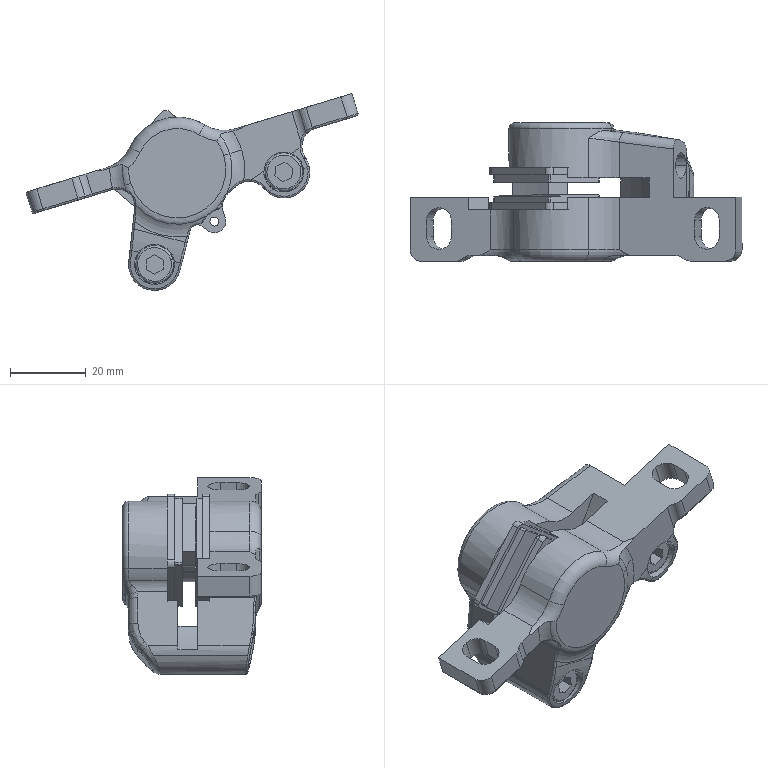Part | SolidWorks | features BaseBody 1 | 1 solid | 275 faces | box 87.761 x 36.6 x 52.032 mm | volume 39694 mm3 | cylinder 100 | plane 98 | spline 46 | torus 29 | cone 2 | commonest cylinder face diameters 1 x19 6 x12 3 x10 5 x9 6.8 x8 10 x8